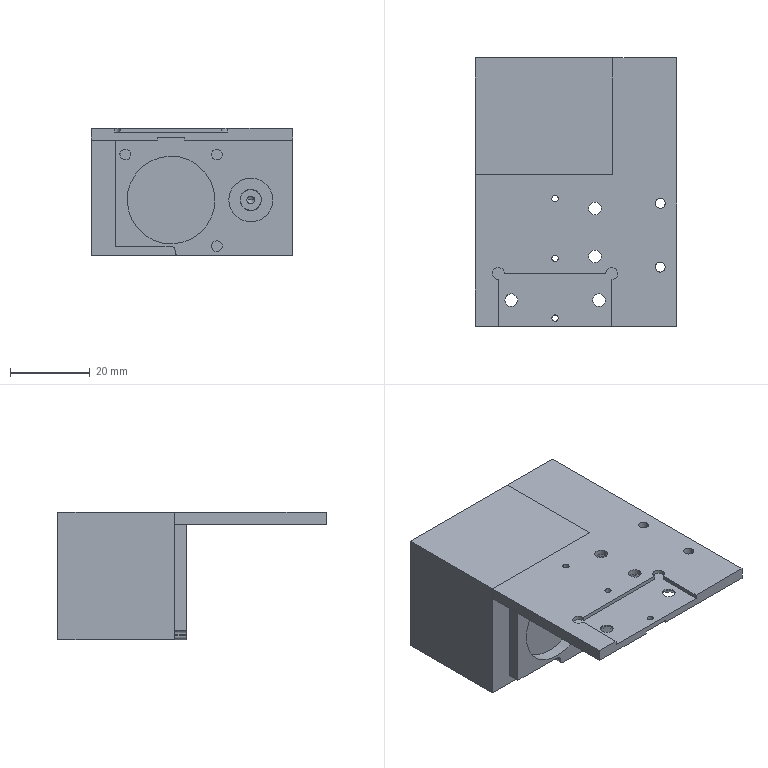NC program | NX | posted with a generic post | part box 50.5 x 67.3 x 32 mm
Whole program:
N10 G17 G21 G94 G90
(PLANAR_MILL_COPY_2_COPY , TOOL : D6A45)
N12 T07 M6
N14 G54
N16 G17 G0 G90 X24.6 Y1.627 B0. C0. S9500 M3
N18 G43 Z30. H7
N20 Z-32.5
N22 G94 G1 Z-35.5 F1250.
N24 X25.443 Y2.334
N26 G3 X25.8 Y3.1 R1.
N28 G1 X21.7
N30 Y-15.9
N32 G2 X20.7 Y-16.9 R1.
N34 G1 X0.1
N36 G2 X-0.9 Y-15.9 R1.
N38 G1 Y15.9
N40 G2 X0.1 Y16.9 R1.
N42 G1 X25.918
N44 G3 X25.769 Y17.732 R1.
N46 G1 X25.278 Y18.432
N48 Z-32.5
N50 G0 Z30.
N52 M5
N54 M2